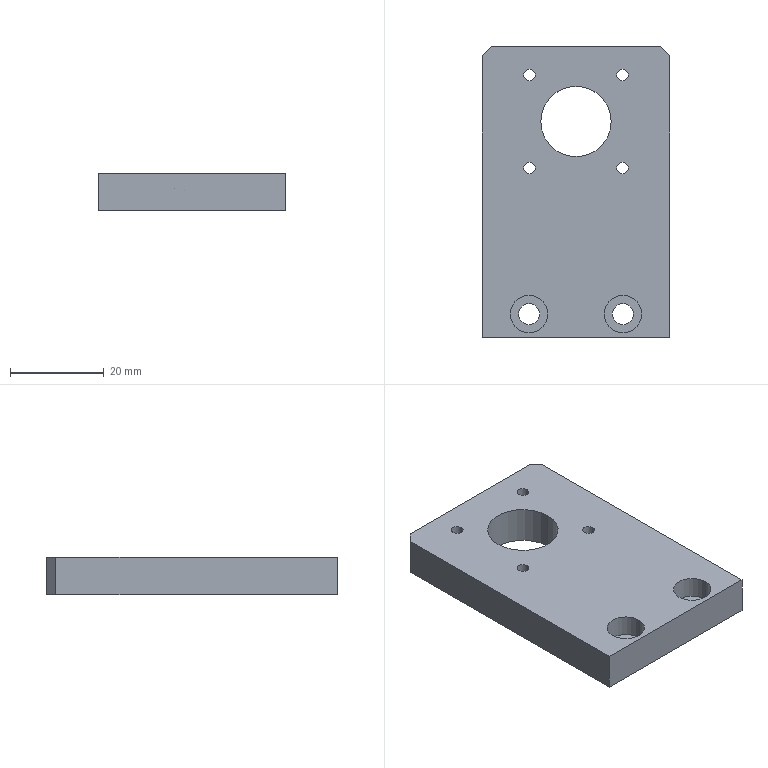Part | STEP file | PN_0007 Mount electronic clip cylinder mounting plate 1 | 1 solid | 28 faces | box 40 x 62 x 8 mm | volume 17667 mm3 | cylinder 18 | plane 10 | commonest cylinder face diameters 2.5 x8 4.5 x4 8 x4 15 x2